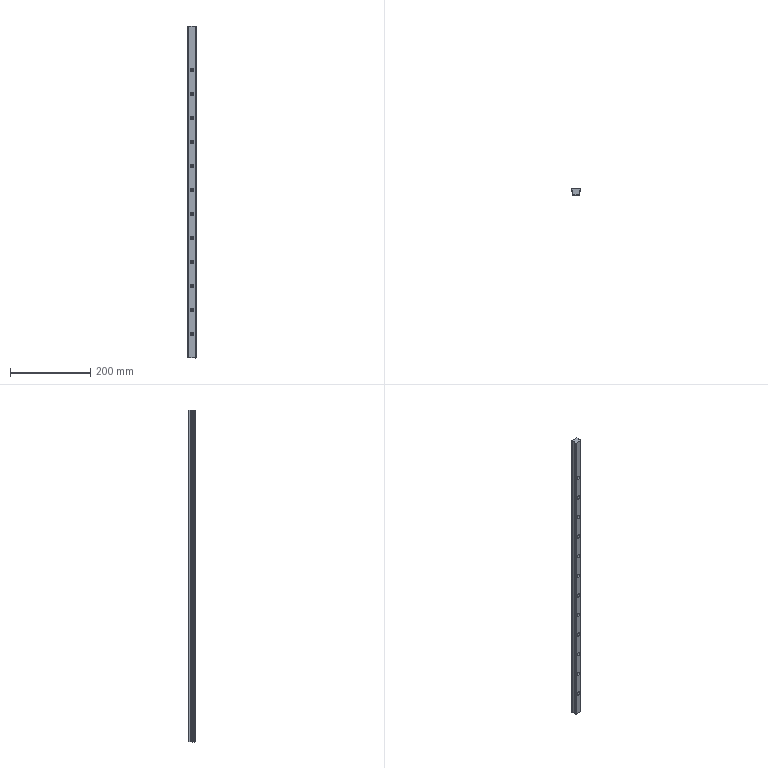Part | SolidWorks | features BaseBody 1 | 1 solid | 77 faces | box 20 x 15.5 x 830 mm | volume 224992 mm3 | cylinder 55 | plane 22 | commonest cylinder face diameters 6 x24 9.5 x24 4.2 x4 5 x3